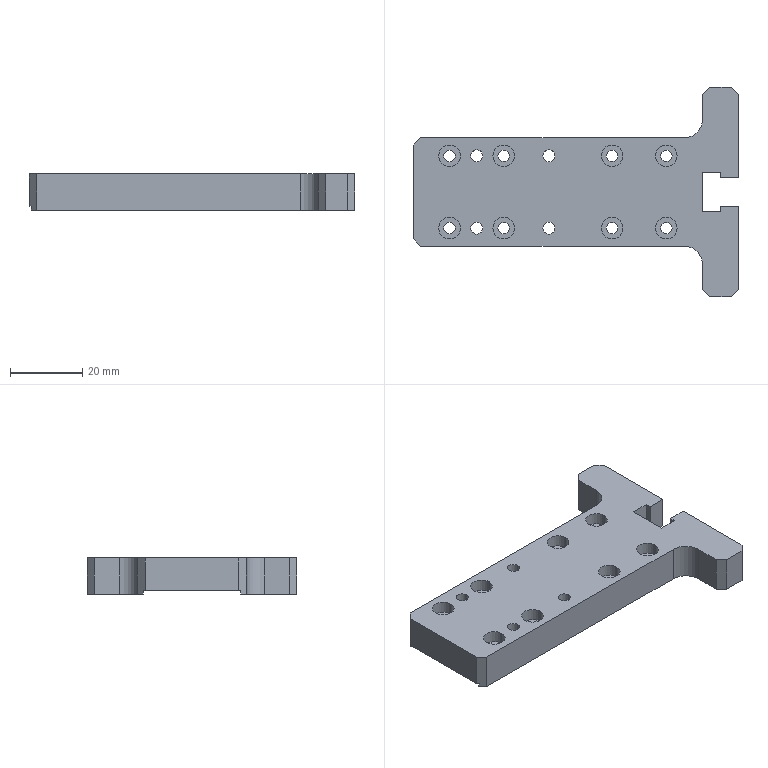Part | STEP file | PN_0054 Mount electronic clip slider mounting plate Z-axis | 1 solid | 78 faces | box 90 x 58 x 10 mm | volume 25065 mm3 | cylinder 42 | plane 36 | commonest cylinder face diameters 3.2 x16 6 x16 3.3 x8 10 x2